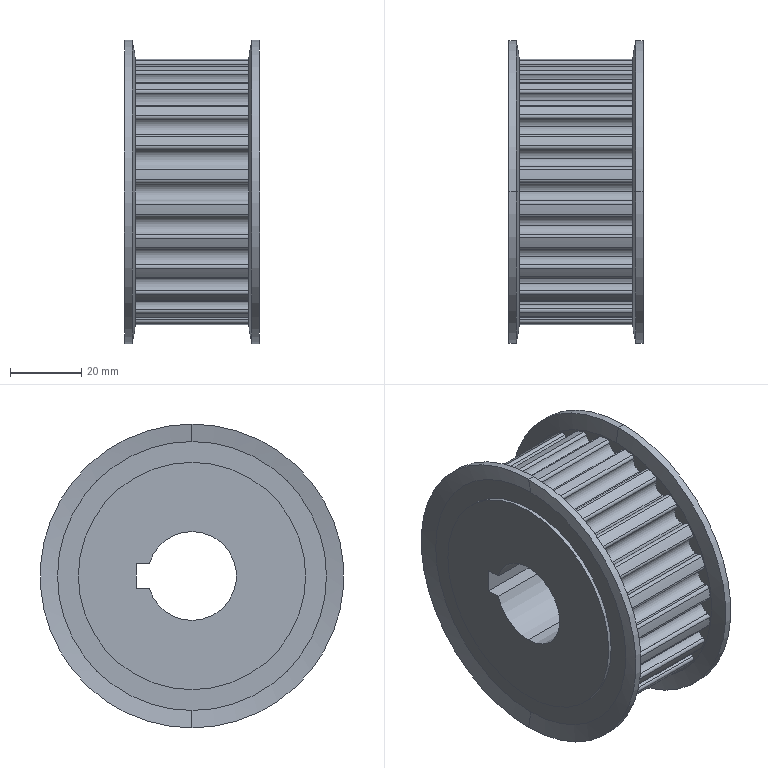Part | SolidWorks | features ICE 2, CirPattern 1, Revolution 1 | 1 solid | 153 faces | box 38 x 85.48 x 85.48 mm | volume 139347 mm3 | cylinder 136 | plane 9 | cone 8 | commonest cylinder face diameters 1.6 x62 5.14 x39 75 x24 64 x4 85.48 x4 25 x3